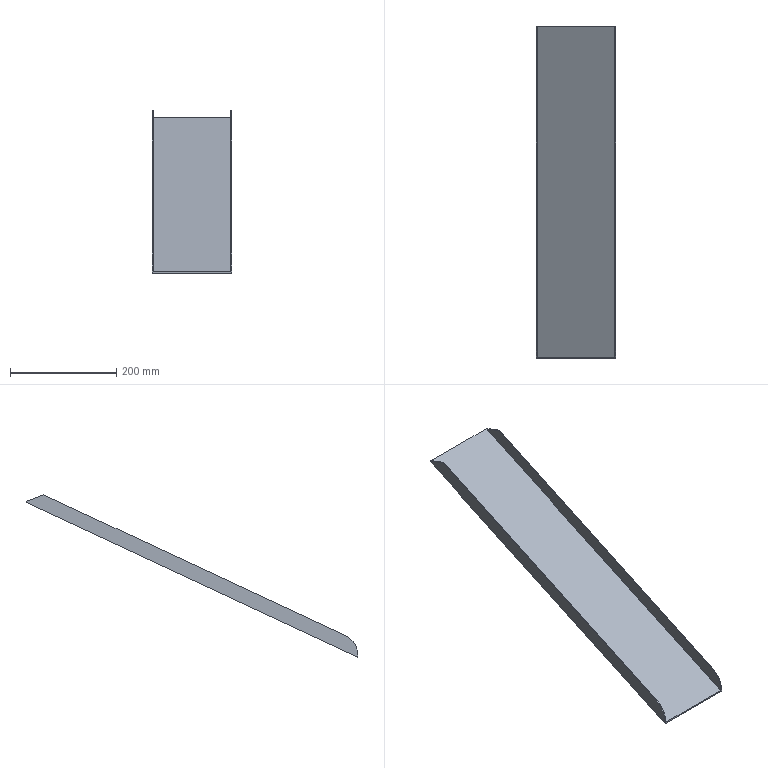Part | NX | features solid 2 | 1 solid | 14 faces | box 150 x 623.143 x 304.875 mm | volume 272745 mm3 | plane 12 | cylinder 2 | commonest cylinder face diameters 80 x2
STEP:
#1=CARTESIAN_POINT('',(-1300.,-690.,-319.111));
#2=VERTEX_POINT('',#1);
#3=CARTESIAN_POINT('',(-1300.,-66.857,-28.534));
#4=VERTEX_POINT('',#3);
#5=CARTESIAN_POINT('',(-1300.,-620.,-286.469));
#6=DIRECTION('',(0.,0.9063,0.4226));
#7=VECTOR('',#6,1000.);
#8=LINE('',#5,#7);
#9=EDGE_CURVE('',#2,#4,#8,.T.);
#10=ORIENTED_EDGE('',*,*,#9,.F.);
#11=CARTESIAN_POINT('',(-1450.,-690.,-319.111));
#12=VERTEX_POINT('',#11);
#13=CARTESIAN_POINT('',(50.,-690.,-319.111));
#14=DIRECTION('',(-1.,0.,0.));
#15=VECTOR('',#14,1000.);
#16=LINE('',#13,#15);
#17=EDGE_CURVE('',#12,#2,#16,.F.);
#18=ORIENTED_EDGE('',*,*,#17,.F.);
#19=CARTESIAN_POINT('',(-1450.,-66.857,-28.534));
#20=VERTEX_POINT('',#19);
#21=CARTESIAN_POINT('',(-1450.,-620.,-286.469));
#22=DIRECTION('',(0.,0.9063,0.4226));
#23=VECTOR('',#22,1000.);
#24=LINE('',#21,#23);
#25=EDGE_CURVE('',#12,#20,#24,.T.);
#26=ORIENTED_EDGE('',*,*,#25,.T.);
#27=CARTESIAN_POINT('',(-1470.,-66.857,-28.534));
#28=DIRECTION('',(-1.,0.,0.));
#29=VECTOR('',#28,1000.);
#30=LINE('',#27,#29);
#31=EDGE_CURVE('',#20,#4,#30,.F.);
#32=ORIENTED_EDGE('',*,*,#31,.T.);
#33=EDGE_LOOP('',(#10,#18,#26,#32));
#34=FACE_BOUND('',#33,.T.);
#35=CARTESIAN_POINT('',(-1470.,-620.,-286.469));
#36=DIRECTION('',(0.,0.4226,-0.9063));
#37=DIRECTION('',(0.,0.9063,0.4226));
#38=AXIS2_PLACEMENT_3D('',#35,#36,#37);
#39=PLANE('',#38);
#40=ADVANCED_FACE('',(#34),#39,.T.);
#41=CARTESIAN_POINT('',(-1300.,-66.857,-26.328));
#42=VERTEX_POINT('',#41);
#43=CARTESIAN_POINT('',(-1300.,-66.857,-180.));
#44=DIRECTION('',(0.,0.,-1.));
#45=VECTOR('',#44,1000.);
#46=LINE('',#43,#45);
#47=EDGE_CURVE('',#4,#42,#46,.F.);
#48=ORIENTED_EDGE('',*,*,#47,.F.);
#49=ORIENTED_EDGE('',*,*,#31,.F.);
#50=CARTESIAN_POINT('',(-1450.,-66.857,-26.328));
#51=VERTEX_POINT('',#50);
#52=CARTESIAN_POINT('',(-1450.,-66.857,-286.469));
#53=DIRECTION('',(0.,0.,-1.));
#54=VECTOR('',#53,1000.);
#55=LINE('',#52,#54);
#56=EDGE_CURVE('',#20,#51,#55,.F.);
#57=ORIENTED_EDGE('',*,*,#56,.T.);
#58=CARTESIAN_POINT('',(-1448.,-66.857,-26.328));
#59=VERTEX_POINT('',#58);
#60=CARTESIAN_POINT('',(-1470.,-66.857,-26.328));
#61=DIRECTION('',(1.,0.,0.));
#62=VECTOR('',#61,1000.);
#63=LINE('',#60,#62);
#64=EDGE_CURVE('',#51,#59,#63,.T.);
#65=ORIENTED_EDGE('',*,*,#64,.T.);
#66=CARTESIAN_POINT('',(-1302.,-66.857,-26.328));
#67=VERTEX_POINT('',#66);
#68=CARTESIAN_POINT('',(-1470.,-66.857,-26.328));
#69=DIRECTION('',(1.,0.,0.));
#70=VECTOR('',#69,1000.);
#71=LINE('',#68,#70);
#72=EDGE_CURVE('',#59,#67,#71,.T.);
#73=ORIENTED_EDGE('',*,*,#72,.T.);
#74=CARTESIAN_POINT('',(-1300.,-66.857,-26.328));
#75=DIRECTION('',(1.,0.,0.));
#76=VECTOR('',#75,1000.);
#77=LINE('',#74,#76);
#78=EDGE_CURVE('',#42,#67,#77,.F.);
#79=ORIENTED_EDGE('',*,*,#78,.F.);
#80=EDGE_LOOP('',(#48,#49,#57,#65,#73,#79));
#81=FACE_BOUND('',#80,.T.);
#82=CARTESIAN_POINT('',(-1470.,-66.857,-180.));
#83=DIRECTION('',(0.,-1.,0.));
#84=DIRECTION('',(1.,0.,0.));
#85=AXIS2_PLACEMENT_3D('',#82,#83,#84);
#86=PLANE('',#85);
#87=ADVANCED_FACE('',(#81),#86,.F.);
#88=CARTESIAN_POINT('',(-1302.,-690.,-316.904));
#89=VERTEX_POINT('',#88);
#90=CARTESIAN_POINT('',(-1302.,-66.857,-26.328));
#91=DIRECTION('',(0.,-0.9063,-0.4226));
#92=VECTOR('',#91,1000.);
#93=LINE('',#90,#92);
#94=EDGE_CURVE('',#67,#89,#93,.T.);
#95=ORIENTED_EDGE('',*,*,#94,.F.);
#96=ORIENTED_EDGE('',*,*,#72,.F.);
#97=CARTESIAN_POINT('',(-1448.,-690.,-316.904));
#98=VERTEX_POINT('',#97);
#99=CARTESIAN_POINT('',(-1448.,-620.845,-284.657));
#100=DIRECTION('',(0.,-0.9063,-0.4226));
#101=VECTOR('',#100,1000.);
#102=LINE('',#99,#101);
#103=EDGE_CURVE('',#98,#59,#102,.F.);
#104=ORIENTED_EDGE('',*,*,#103,.F.);
#105=CARTESIAN_POINT('',(-1470.,-690.,-316.904));
#106=DIRECTION('',(1.,0.,0.));
#107=VECTOR('',#106,1000.);
#108=LINE('',#105,#107);
#109=EDGE_CURVE('',#98,#89,#108,.T.);
#110=ORIENTED_EDGE('',*,*,#109,.T.);
#111=EDGE_LOOP('',(#95,#96,#104,#110));
#112=FACE_BOUND('',#111,.T.);
#113=CARTESIAN_POINT('',(-1470.,-620.845,-284.657));
#114=DIRECTION('',(0.,0.4226,-0.9063));
#115=DIRECTION('',(0.,0.9063,0.4226));
#116=AXIS2_PLACEMENT_3D('',#113,#114,#115);
#117=PLANE('',#116);
#118=ADVANCED_FACE('',(#112),#117,.F.);
#119=CARTESIAN_POINT('',(-1300.,-690.,-314.802));
#120=VERTEX_POINT('',#119);
#121=CARTESIAN_POINT('',(-1300.,-690.,-570.));
#122=DIRECTION('',(0.,0.,1.));
#123=VECTOR('',#122,1000.);
#124=LINE('',#121,#123);
#125=EDGE_CURVE('',#120,#2,#124,.F.);
#126=ORIENTED_EDGE('',*,*,#125,.F.);
#127=CARTESIAN_POINT('',(-1302.,-690.,-314.802));
#128=VERTEX_POINT('',#127);
#129=CARTESIAN_POINT('',(-1302.,-690.,-314.802));
#130=DIRECTION('',(-1.,0.,0.));
#131=VECTOR('',#130,1000.);
#132=LINE('',#129,#131);
#133=EDGE_CURVE('',#120,#128,#132,.T.);
#134=ORIENTED_EDGE('',*,*,#133,.T.);
#135=CARTESIAN_POINT('',(-1302.,-690.,-570.));
#136=DIRECTION('',(0.,0.,1.));
#137=VECTOR('',#136,1000.);
#138=LINE('',#135,#137);
#139=EDGE_CURVE('',#89,#128,#138,.T.);
#140=ORIENTED_EDGE('',*,*,#139,.F.);
#141=ORIENTED_EDGE('',*,*,#109,.F.);
#142=CARTESIAN_POINT('',(-1448.,-690.,-314.802));
#143=VERTEX_POINT('',#142);
#144=CARTESIAN_POINT('',(-1448.,-690.,-570.));
#145=DIRECTION('',(0.,0.,-1.));
#146=VECTOR('',#145,1000.);
#147=LINE('',#144,#146);
#148=EDGE_CURVE('',#98,#143,#147,.F.);
#149=ORIENTED_EDGE('',*,*,#148,.T.);
#150=CARTESIAN_POINT('',(-1450.,-690.,-314.802));
#151=VERTEX_POINT('',#150);
#152=CARTESIAN_POINT('',(50.,-690.,-314.802));
#153=DIRECTION('',(-1.,0.,0.));
#154=VECTOR('',#153,1000.);
#155=LINE('',#152,#154);
#156=EDGE_CURVE('',#143,#151,#155,.T.);
#157=ORIENTED_EDGE('',*,*,#156,.T.);
#158=CARTESIAN_POINT('',(-1450.,-690.,-570.));
#159=DIRECTION('',(0.,0.,-1.));
#160=VECTOR('',#159,1000.);
#161=LINE('',#158,#160);
#162=EDGE_CURVE('',#12,#151,#161,.F.);
#163=ORIENTED_EDGE('',*,*,#162,.F.);
#164=ORIENTED_EDGE('',*,*,#17,.T.);
#165=EDGE_LOOP('',(#126,#134,#140,#141,#149,#157,#163,#164));
#166=FACE_BOUND('',#165,.T.);
#167=CARTESIAN_POINT('',(50.,-690.,-570.));
#168=DIRECTION('',(0.,1.,0.));
#169=DIRECTION('',(-1.,0.,0.));
#170=AXIS2_PLACEMENT_3D('',#167,#168,#169);
#171=PLANE('',#170);
#172=ADVANCED_FACE('',(#166),#171,.F.);
#173=CARTESIAN_POINT('',(-1450.,-666.905,-278.55));
#174=VERTEX_POINT('',#173);
#175=CARTESIAN_POINT('',(-1450.,-100.08,-14.235));
#176=VERTEX_POINT('',#175);
#177=CARTESIAN_POINT('',(-1450.,-700.565,-294.246));
#178=DIRECTION('',(0.,-0.9063,-0.4226));
#179=VECTOR('',#178,1000.);
#180=LINE('',#177,#179);
#181=EDGE_CURVE('',#174,#176,#180,.F.);
#182=ORIENTED_EDGE('',*,*,#181,.T.);
#183=CARTESIAN_POINT('',(-1450.,-66.857,-26.328));
#184=DIRECTION('',(0.,0.9397,-0.342));
#185=VECTOR('',#184,1000.);
#186=LINE('',#183,#185);
#187=EDGE_CURVE('',#176,#51,#186,.T.);
#188=ORIENTED_EDGE('',*,*,#187,.T.);
#189=ORIENTED_EDGE('',*,*,#56,.F.);
#190=ORIENTED_EDGE('',*,*,#25,.F.);
#191=ORIENTED_EDGE('',*,*,#162,.T.);
#192=CARTESIAN_POINT('',(-1450.,-650.,-314.802));
#193=DIRECTION('',(1.,0.,0.));
#194=DIRECTION('',(0.,0.,-1.));
#195=AXIS2_PLACEMENT_3D('',#192,#193,#194);
#196=CIRCLE('',#195,40.);
#197=EDGE_CURVE('',#151,#174,#196,.F.);
#198=ORIENTED_EDGE('',*,*,#197,.T.);
#199=EDGE_LOOP('',(#182,#188,#189,#190,#191,#198));
#200=FACE_BOUND('',#199,.T.);
#201=CARTESIAN_POINT('',(-1450.,-620.,-286.469));
#202=DIRECTION('',(1.,0.,0.));
#203=DIRECTION('',(0.,0.,-1.));
#204=AXIS2_PLACEMENT_3D('',#201,#202,#203);
#205=PLANE('',#204);
#206=ADVANCED_FACE('',(#200),#205,.F.);
#207=ORIENTED_EDGE('',*,*,#47,.T.);
#208=CARTESIAN_POINT('',(-1300.,-100.08,-14.235));
#209=VERTEX_POINT('',#208);
#210=CARTESIAN_POINT('',(-1300.,-100.08,-14.235));
#211=DIRECTION('',(0.,0.9397,-0.342));
#212=VECTOR('',#211,1000.);
#213=LINE('',#210,#212);
#214=EDGE_CURVE('',#42,#209,#213,.F.);
#215=ORIENTED_EDGE('',*,*,#214,.T.);
#216=CARTESIAN_POINT('',(-1300.,-666.905,-278.55));
#217=VERTEX_POINT('',#216);
#218=CARTESIAN_POINT('',(-1300.,-77.423,-3.67));
#219=DIRECTION('',(0.,-0.9063,-0.4226));
#220=VECTOR('',#219,1000.);
#221=LINE('',#218,#220);
#222=EDGE_CURVE('',#209,#217,#221,.T.);
#223=ORIENTED_EDGE('',*,*,#222,.T.);
#224=CARTESIAN_POINT('',(-1300.,-650.,-314.802));
#225=DIRECTION('',(-1.,0.,0.));
#226=DIRECTION('',(0.,0.,1.));
#227=AXIS2_PLACEMENT_3D('',#224,#225,#226);
#228=CIRCLE('',#227,40.);
#229=EDGE_CURVE('',#217,#120,#228,.F.);
#230=ORIENTED_EDGE('',*,*,#229,.T.);
#231=ORIENTED_EDGE('',*,*,#125,.T.);
#232=ORIENTED_EDGE('',*,*,#9,.T.);
#233=EDGE_LOOP('',(#207,#215,#223,#230,#231,#232));
#234=FACE_BOUND('',#233,.T.);
#235=CARTESIAN_POINT('',(-1300.,-40.,0.));
#236=DIRECTION('',(-1.,0.,0.));
#237=DIRECTION('',(0.,0.,1.));
#238=AXIS2_PLACEMENT_3D('',#235,#236,#237);
#239=PLANE('',#238);
#240=ADVANCED_FACE('',(#234),#239,.F.);
#241=CARTESIAN_POINT('',(-1448.,-666.905,-278.55));
#242=VERTEX_POINT('',#241);
#243=CARTESIAN_POINT('',(-1448.,-100.08,-14.235));
#244=VERTEX_POINT('',#243);
#245=CARTESIAN_POINT('',(-1448.,-700.565,-294.246));
#246=DIRECTION('',(0.,-0.9063,-0.4226));
#247=VECTOR('',#246,1000.);
#248=LINE('',#245,#247);
#249=EDGE_CURVE('',#242,#244,#248,.F.);
#250=ORIENTED_EDGE('',*,*,#249,.T.);
#251=CARTESIAN_POINT('',(-1470.,-100.08,-14.235));
#252=DIRECTION('',(1.,0.,0.));
#253=VECTOR('',#252,1000.);
#254=LINE('',#251,#253);
#255=EDGE_CURVE('',#244,#176,#254,.F.);
#256=ORIENTED_EDGE('',*,*,#255,.T.);
#257=ORIENTED_EDGE('',*,*,#181,.F.);
#258=CARTESIAN_POINT('',(-1470.,-666.905,-278.55));
#259=DIRECTION('',(-1.,0.,0.));
#260=VECTOR('',#259,1000.);
#261=LINE('',#258,#260);
#262=EDGE_CURVE('',#174,#242,#261,.F.);
#263=ORIENTED_EDGE('',*,*,#262,.T.);
#264=EDGE_LOOP('',(#250,#256,#257,#263));
#265=FACE_BOUND('',#264,.T.);
#266=CARTESIAN_POINT('',(-1470.,-700.565,-294.246));
#267=DIRECTION('',(0.,0.4226,-0.9063));
#268=DIRECTION('',(0.,0.9063,0.4226));
#269=AXIS2_PLACEMENT_3D('',#266,#267,#268);
#270=PLANE('',#269);
#271=ADVANCED_FACE('',(#265),#270,.F.);
#272=ORIENTED_EDGE('',*,*,#103,.T.);
#273=CARTESIAN_POINT('',(-1448.,-523.717,139.956));
#274=DIRECTION('',(0.,-0.9397,0.342));
#275=VECTOR('',#274,1000.);
#276=LINE('',#273,#275);
#277=EDGE_CURVE('',#59,#244,#276,.T.);
#278=ORIENTED_EDGE('',*,*,#277,.T.);
#279=ORIENTED_EDGE('',*,*,#249,.F.);
#280=CARTESIAN_POINT('',(-1448.,-650.,-314.802));
#281=DIRECTION('',(1.,0.,0.));
#282=DIRECTION('',(0.,0.,-1.));
#283=AXIS2_PLACEMENT_3D('',#280,#281,#282);
#284=CIRCLE('',#283,40.);
#285=EDGE_CURVE('',#242,#143,#284,.T.);
#286=ORIENTED_EDGE('',*,*,#285,.T.);
#287=ORIENTED_EDGE('',*,*,#148,.F.);
#288=EDGE_LOOP('',(#272,#278,#279,#286,#287));
#289=FACE_BOUND('',#288,.T.);
#290=CARTESIAN_POINT('',(-1448.,-690.,-316.904));
#291=DIRECTION('',(1.,0.,0.));
#292=DIRECTION('',(0.,0.,-1.));
#293=AXIS2_PLACEMENT_3D('',#290,#291,#292);
#294=PLANE('',#293);
#295=ADVANCED_FACE('',(#289),#294,.T.);
#296=ORIENTED_EDGE('',*,*,#222,.F.);
#297=CARTESIAN_POINT('',(-1302.,-100.08,-14.235));
#298=VERTEX_POINT('',#297);
#299=CARTESIAN_POINT('',(-1300.,-100.08,-14.235));
#300=DIRECTION('',(-1.,0.,0.));
#301=VECTOR('',#300,1000.);
#302=LINE('',#299,#301);
#303=EDGE_CURVE('',#209,#298,#302,.T.);
#304=ORIENTED_EDGE('',*,*,#303,.T.);
#305=CARTESIAN_POINT('',(-1302.,-666.905,-278.55));
#306=VERTEX_POINT('',#305);
#307=CARTESIAN_POINT('',(-1302.,-77.423,-3.67));
#308=DIRECTION('',(0.,-0.9063,-0.4226));
#309=VECTOR('',#308,1000.);
#310=LINE('',#307,#309);
#311=EDGE_CURVE('',#298,#306,#310,.T.);
#312=ORIENTED_EDGE('',*,*,#311,.T.);
#313=CARTESIAN_POINT('',(-1300.,-666.905,-278.55));
#314=DIRECTION('',(1.,0.,0.));
#315=VECTOR('',#314,1000.);
#316=LINE('',#313,#315);
#317=EDGE_CURVE('',#306,#217,#316,.T.);
#318=ORIENTED_EDGE('',*,*,#317,.T.);
#319=EDGE_LOOP('',(#296,#304,#312,#318));
#320=FACE_BOUND('',#319,.T.);
#321=CARTESIAN_POINT('',(-1300.,-77.423,-3.67));
#322=DIRECTION('',(0.,0.4226,-0.9063));
#323=DIRECTION('',(0.,-0.9063,-0.4226));
#324=AXIS2_PLACEMENT_3D('',#321,#322,#323);
#325=PLANE('',#324);
#326=ADVANCED_FACE('',(#320),#325,.F.);
#327=ORIENTED_EDGE('',*,*,#311,.F.);
#328=CARTESIAN_POINT('',(-1302.,-66.857,-26.328));
#329=DIRECTION('',(0.,-0.9397,0.342));
#330=VECTOR('',#329,1000.);
#331=LINE('',#328,#330);
#332=EDGE_CURVE('',#298,#67,#331,.F.);
#333=ORIENTED_EDGE('',*,*,#332,.T.);
#334=ORIENTED_EDGE('',*,*,#94,.T.);
#335=ORIENTED_EDGE('',*,*,#139,.T.);
#336=CARTESIAN_POINT('',(-1302.,-650.,-314.802));
#337=DIRECTION('',(-1.,0.,0.));
#338=DIRECTION('',(0.,0.,1.));
#339=AXIS2_PLACEMENT_3D('',#336,#337,#338);
#340=CIRCLE('',#339,40.);
#341=EDGE_CURVE('',#128,#306,#340,.T.);
#342=ORIENTED_EDGE('',*,*,#341,.T.);
#343=EDGE_LOOP('',(#327,#333,#334,#335,#342));
#344=FACE_BOUND('',#343,.T.);
#345=CARTESIAN_POINT('',(-1302.,-66.857,-26.328));
#346=DIRECTION('',(-1.,0.,0.));
#347=DIRECTION('',(0.,0.,1.));
#348=AXIS2_PLACEMENT_3D('',#345,#346,#347);
#349=PLANE('',#348);
#350=ADVANCED_FACE('',(#344),#349,.T.);
#351=ORIENTED_EDGE('',*,*,#229,.F.);
#352=ORIENTED_EDGE('',*,*,#317,.F.);
#353=ORIENTED_EDGE('',*,*,#341,.F.);
#354=ORIENTED_EDGE('',*,*,#133,.F.);
#355=EDGE_LOOP('',(#351,#352,#353,#354));
#356=FACE_BOUND('',#355,.T.);
#357=CARTESIAN_POINT('',(50.,-650.,-314.802));
#358=DIRECTION('',(-1.,0.,0.));
#359=DIRECTION('',(0.,0.,1.));
#360=AXIS2_PLACEMENT_3D('',#357,#358,#359);
#361=CYLINDRICAL_SURFACE('',#360,40.);
#362=ADVANCED_FACE('',(#356),#361,.T.);
#363=ORIENTED_EDGE('',*,*,#197,.F.);
#364=ORIENTED_EDGE('',*,*,#156,.F.);
#365=ORIENTED_EDGE('',*,*,#285,.F.);
#366=ORIENTED_EDGE('',*,*,#262,.F.);
#367=EDGE_LOOP('',(#363,#364,#365,#366));
#368=FACE_BOUND('',#367,.T.);
#369=CARTESIAN_POINT('',(-1470.,-650.,-314.802));
#370=DIRECTION('',(1.,0.,0.));
#371=DIRECTION('',(0.,0.,-1.));
#372=AXIS2_PLACEMENT_3D('',#369,#370,#371);
#373=CYLINDRICAL_SURFACE('',#372,40.);
#374=ADVANCED_FACE('',(#368),#373,.T.);
#375=ORIENTED_EDGE('',*,*,#187,.F.);
#376=ORIENTED_EDGE('',*,*,#255,.F.);
#377=ORIENTED_EDGE('',*,*,#277,.F.);
#378=ORIENTED_EDGE('',*,*,#64,.F.);
#379=EDGE_LOOP('',(#375,#376,#377,#378));
#380=FACE_BOUND('',#379,.T.);
#381=CARTESIAN_POINT('',(-1470.,-66.857,-26.328));
#382=DIRECTION('',(0.,0.342,0.9397));
#383=DIRECTION('',(0.,-0.9397,0.342));
#384=AXIS2_PLACEMENT_3D('',#381,#382,#383);
#385=PLANE('',#384);
#386=ADVANCED_FACE('',(#380),#385,.T.);
#387=ORIENTED_EDGE('',*,*,#214,.F.);
#388=ORIENTED_EDGE('',*,*,#78,.T.);
#389=ORIENTED_EDGE('',*,*,#332,.F.);
#390=ORIENTED_EDGE('',*,*,#303,.F.);
#391=EDGE_LOOP('',(#387,#388,#389,#390));
#392=FACE_BOUND('',#391,.T.);
#393=CARTESIAN_POINT('',(-1300.,-100.08,-14.235));
#394=DIRECTION('',(0.,-0.342,-0.9397));
#395=DIRECTION('',(0.,0.9397,-0.342));
#396=AXIS2_PLACEMENT_3D('',#393,#394,#395);
#397=PLANE('',#396);
#398=ADVANCED_FACE('',(#392),#397,.F.);
#399=CLOSED_SHELL('',(#40,#87,#118,#172,#206,#240,#271,#295,#326,#350,#362,#374,#386,#398));
#400=MANIFOLD_SOLID_BREP('',#399);
#401=(LENGTH_UNIT()NAMED_UNIT(*)SI_UNIT(.MILLI.,.METRE.));
#402=UNCERTAINTY_MEASURE_WITH_UNIT(LENGTH_MEASURE(0.00001),#401,'','');
#403=(NAMED_UNIT(*)PLANE_ANGLE_UNIT()SI_UNIT($,.RADIAN.));
#404=(NAMED_UNIT(*)SI_UNIT($,.STERADIAN.)SOLID_ANGLE_UNIT());
#405=(GEOMETRIC_REPRESENTATION_CONTEXT(3)GLOBAL_UNCERTAINTY_ASSIGNED_CONTEXT((#402))GLOBAL_UNIT_ASSIGNED_CONTEXT((#401,#403,#404))REPRESENTATION_CONTEXT('',''));
#406=ADVANCED_BREP_SHAPE_REPRESENTATION('',(#400),#405);